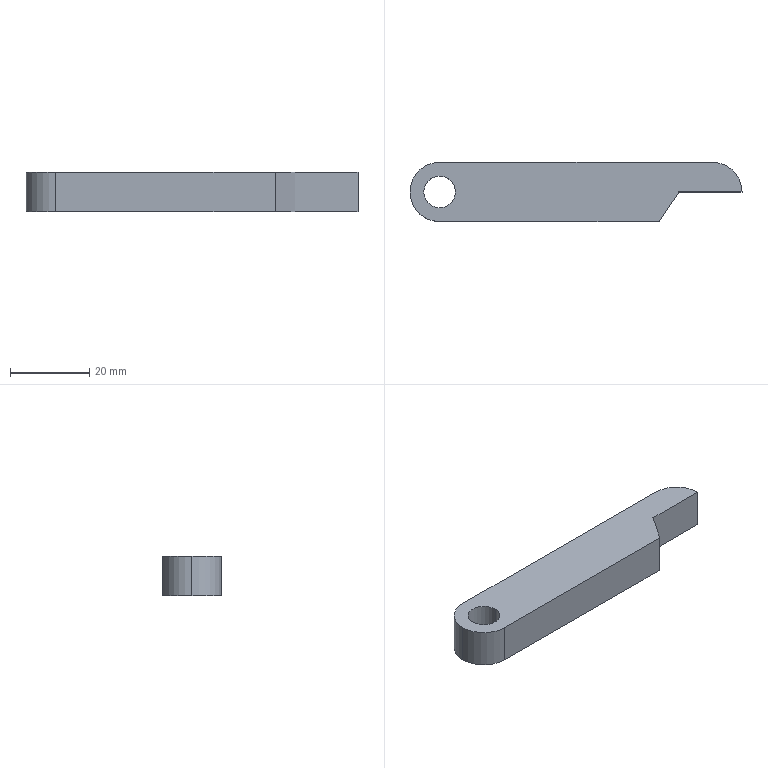Part | SolidWorks | features Extrusion 1 | 1 solid | 11 faces | box 84 x 15 x 10 mm | volume 10349 mm3 | plane 6 | cylinder 5 | commonest cylinder face diameters 15 x3 8 x2
STEP:
#1=CARTESIAN_POINT('',(-4.,0.,10.));
#2=VERTEX_POINT('',#1);
#3=CARTESIAN_POINT('',(4.,0.,10.));
#4=VERTEX_POINT('',#3);
#5=CARTESIAN_POINT('',(0.,0.,10.));
#6=DIRECTION('',(0.,0.,1.));
#7=DIRECTION('',(1.,0.,0.));
#8=AXIS2_PLACEMENT_3D('',#5,#6,#7);
#9=CIRCLE('',#8,4.);
#10=EDGE_CURVE('',#2,#4,#9,.T.);
#11=ORIENTED_EDGE('',*,*,#10,.T.);
#12=CARTESIAN_POINT('',(4.,0.,0.));
#13=VERTEX_POINT('',#12);
#14=CARTESIAN_POINT('',(4.,0.,10.));
#15=DIRECTION('',(0.,0.,-1.));
#16=VECTOR('',#15,1000.);
#17=LINE('',#14,#16);
#18=EDGE_CURVE('',#4,#13,#17,.T.);
#19=ORIENTED_EDGE('',*,*,#18,.T.);
#20=CARTESIAN_POINT('',(-4.,0.,0.));
#21=VERTEX_POINT('',#20);
#22=CARTESIAN_POINT('',(0.,0.,0.));
#23=DIRECTION('',(0.,0.,1.));
#24=DIRECTION('',(1.,0.,0.));
#25=AXIS2_PLACEMENT_3D('',#22,#23,#24);
#26=CIRCLE('',#25,4.);
#27=EDGE_CURVE('',#21,#13,#26,.T.);
#28=ORIENTED_EDGE('',*,*,#27,.F.);
#29=CARTESIAN_POINT('',(-4.,0.,10.));
#30=DIRECTION('',(0.,0.,-1.));
#31=VECTOR('',#30,1000.);
#32=LINE('',#29,#31);
#33=EDGE_CURVE('',#2,#21,#32,.T.);
#34=ORIENTED_EDGE('',*,*,#33,.F.);
#35=EDGE_LOOP('',(#11,#19,#28,#34));
#36=FACE_OUTER_BOUND('',#35,.T.);
#37=CARTESIAN_POINT('',(0.,0.,10.));
#38=DIRECTION('',(0.,0.,-1.));
#39=DIRECTION('',(-1.,0.,0.));
#40=AXIS2_PLACEMENT_3D('',#37,#38,#39);
#41=CYLINDRICAL_SURFACE('',#40,4.);
#42=ADVANCED_FACE('',(#36),#41,.F.);
#43=CARTESIAN_POINT('',(-7.5,0.,10.));
#44=VERTEX_POINT('',#43);
#45=CARTESIAN_POINT('',(0.,-7.5,10.));
#46=VERTEX_POINT('',#45);
#47=CARTESIAN_POINT('',(0.,0.,10.));
#48=DIRECTION('',(0.,0.,1.));
#49=DIRECTION('',(1.,0.,0.));
#50=AXIS2_PLACEMENT_3D('',#47,#48,#49);
#51=CIRCLE('',#50,7.5);
#52=EDGE_CURVE('',#44,#46,#51,.T.);
#53=ORIENTED_EDGE('',*,*,#52,.F.);
#54=CARTESIAN_POINT('',(-7.5,0.,0.));
#55=VERTEX_POINT('',#54);
#56=CARTESIAN_POINT('',(-7.5,0.,10.));
#57=DIRECTION('',(0.,0.,-1.));
#58=VECTOR('',#57,1000.);
#59=LINE('',#56,#58);
#60=EDGE_CURVE('',#44,#55,#59,.T.);
#61=ORIENTED_EDGE('',*,*,#60,.T.);
#62=CARTESIAN_POINT('',(0.,-7.5,0.));
#63=VERTEX_POINT('',#62);
#64=CARTESIAN_POINT('',(0.,0.,0.));
#65=DIRECTION('',(0.,0.,1.));
#66=DIRECTION('',(1.,0.,0.));
#67=AXIS2_PLACEMENT_3D('',#64,#65,#66);
#68=CIRCLE('',#67,7.5);
#69=EDGE_CURVE('',#55,#63,#68,.T.);
#70=ORIENTED_EDGE('',*,*,#69,.T.);
#71=CARTESIAN_POINT('',(0.,-7.5,10.));
#72=DIRECTION('',(0.,0.,-1.));
#73=VECTOR('',#72,1000.);
#74=LINE('',#71,#73);
#75=EDGE_CURVE('',#46,#63,#74,.T.);
#76=ORIENTED_EDGE('',*,*,#75,.F.);
#77=EDGE_LOOP('',(#53,#61,#70,#76));
#78=FACE_OUTER_BOUND('',#77,.T.);
#79=CARTESIAN_POINT('',(0.,0.,10.));
#80=DIRECTION('',(0.,0.,-1.));
#81=DIRECTION('',(-1.,0.,0.));
#82=AXIS2_PLACEMENT_3D('',#79,#80,#81);
#83=CYLINDRICAL_SURFACE('',#82,7.5);
#84=ADVANCED_FACE('',(#78),#83,.T.);
#85=CARTESIAN_POINT('',(55.536,-7.5,10.));
#86=VERTEX_POINT('',#85);
#87=CARTESIAN_POINT('',(60.5,0.,10.));
#88=VERTEX_POINT('',#87);
#89=CARTESIAN_POINT('',(55.536,-7.5,10.));
#90=DIRECTION('',(0.552,0.8339,0.));
#91=VECTOR('',#90,1000.);
#92=LINE('',#89,#91);
#93=EDGE_CURVE('',#86,#88,#92,.T.);
#94=ORIENTED_EDGE('',*,*,#93,.T.);
#95=CARTESIAN_POINT('',(76.5,0.,10.));
#96=VERTEX_POINT('',#95);
#97=CARTESIAN_POINT('',(60.5,0.,10.));
#98=DIRECTION('',(1.,0.,0.));
#99=VECTOR('',#98,1000.);
#100=LINE('',#97,#99);
#101=EDGE_CURVE('',#88,#96,#100,.T.);
#102=ORIENTED_EDGE('',*,*,#101,.T.);
#103=CARTESIAN_POINT('',(69.,7.5,10.));
#104=VERTEX_POINT('',#103);
#105=CARTESIAN_POINT('',(69.,0.,10.));
#106=DIRECTION('',(0.,0.,1.));
#107=DIRECTION('',(1.,0.,0.));
#108=AXIS2_PLACEMENT_3D('',#105,#106,#107);
#109=CIRCLE('',#108,7.5);
#110=EDGE_CURVE('',#96,#104,#109,.T.);
#111=ORIENTED_EDGE('',*,*,#110,.T.);
#112=CARTESIAN_POINT('',(0.,7.5,10.));
#113=VERTEX_POINT('',#112);
#114=CARTESIAN_POINT('',(0.,7.5,10.));
#115=DIRECTION('',(-1.,0.,0.));
#116=VECTOR('',#115,1000.);
#117=LINE('',#114,#116);
#118=EDGE_CURVE('',#104,#113,#117,.T.);
#119=ORIENTED_EDGE('',*,*,#118,.T.);
#120=CARTESIAN_POINT('',(0.,0.,10.));
#121=DIRECTION('',(0.,0.,1.));
#122=DIRECTION('',(1.,0.,0.));
#123=AXIS2_PLACEMENT_3D('',#120,#121,#122);
#124=CIRCLE('',#123,7.5);
#125=EDGE_CURVE('',#113,#44,#124,.T.);
#126=ORIENTED_EDGE('',*,*,#125,.T.);
#127=ORIENTED_EDGE('',*,*,#52,.T.);
#128=CARTESIAN_POINT('',(55.536,-7.5,10.));
#129=DIRECTION('',(1.,0.,0.));
#130=VECTOR('',#129,1000.);
#131=LINE('',#128,#130);
#132=EDGE_CURVE('',#46,#86,#131,.T.);
#133=ORIENTED_EDGE('',*,*,#132,.T.);
#134=EDGE_LOOP('',(#94,#102,#111,#119,#126,#127,#133));
#135=FACE_OUTER_BOUND('',#134,.T.);
#136=ORIENTED_EDGE('',*,*,#10,.F.);
#137=CARTESIAN_POINT('',(0.,0.,10.));
#138=DIRECTION('',(0.,0.,1.));
#139=DIRECTION('',(1.,0.,0.));
#140=AXIS2_PLACEMENT_3D('',#137,#138,#139);
#141=CIRCLE('',#140,4.);
#142=EDGE_CURVE('',#4,#2,#141,.T.);
#143=ORIENTED_EDGE('',*,*,#142,.F.);
#144=EDGE_LOOP('',(#136,#143));
#145=FACE_BOUND('',#144,.T.);
#146=CARTESIAN_POINT('',(69.,0.,10.));
#147=DIRECTION('',(0.,0.,1.));
#148=DIRECTION('',(1.,0.,0.));
#149=AXIS2_PLACEMENT_3D('',#146,#147,#148);
#150=PLANE('',#149);
#151=ADVANCED_FACE('',(#135,#145),#150,.T.);
#152=CARTESIAN_POINT('',(55.536,-7.5,0.));
#153=VERTEX_POINT('',#152);
#154=CARTESIAN_POINT('',(60.5,0.,0.));
#155=VERTEX_POINT('',#154);
#156=CARTESIAN_POINT('',(55.536,-7.5,0.));
#157=DIRECTION('',(0.552,0.8339,0.));
#158=VECTOR('',#157,1000.);
#159=LINE('',#156,#158);
#160=EDGE_CURVE('',#153,#155,#159,.T.);
#161=ORIENTED_EDGE('',*,*,#160,.F.);
#162=CARTESIAN_POINT('',(55.536,-7.5,0.));
#163=DIRECTION('',(1.,0.,0.));
#164=VECTOR('',#163,1000.);
#165=LINE('',#162,#164);
#166=EDGE_CURVE('',#63,#153,#165,.T.);
#167=ORIENTED_EDGE('',*,*,#166,.F.);
#168=ORIENTED_EDGE('',*,*,#69,.F.);
#169=CARTESIAN_POINT('',(0.,7.5,0.));
#170=VERTEX_POINT('',#169);
#171=CARTESIAN_POINT('',(0.,0.,0.));
#172=DIRECTION('',(0.,0.,1.));
#173=DIRECTION('',(1.,0.,0.));
#174=AXIS2_PLACEMENT_3D('',#171,#172,#173);
#175=CIRCLE('',#174,7.5);
#176=EDGE_CURVE('',#170,#55,#175,.T.);
#177=ORIENTED_EDGE('',*,*,#176,.F.);
#178=CARTESIAN_POINT('',(69.,7.5,0.));
#179=VERTEX_POINT('',#178);
#180=CARTESIAN_POINT('',(0.,7.5,0.));
#181=DIRECTION('',(-1.,0.,0.));
#182=VECTOR('',#181,1000.);
#183=LINE('',#180,#182);
#184=EDGE_CURVE('',#179,#170,#183,.T.);
#185=ORIENTED_EDGE('',*,*,#184,.F.);
#186=CARTESIAN_POINT('',(76.5,0.,0.));
#187=VERTEX_POINT('',#186);
#188=CARTESIAN_POINT('',(69.,0.,0.));
#189=DIRECTION('',(0.,0.,1.));
#190=DIRECTION('',(1.,0.,0.));
#191=AXIS2_PLACEMENT_3D('',#188,#189,#190);
#192=CIRCLE('',#191,7.5);
#193=EDGE_CURVE('',#187,#179,#192,.T.);
#194=ORIENTED_EDGE('',*,*,#193,.F.);
#195=CARTESIAN_POINT('',(60.5,0.,0.));
#196=DIRECTION('',(1.,0.,0.));
#197=VECTOR('',#196,1000.);
#198=LINE('',#195,#197);
#199=EDGE_CURVE('',#155,#187,#198,.T.);
#200=ORIENTED_EDGE('',*,*,#199,.F.);
#201=EDGE_LOOP('',(#161,#167,#168,#177,#185,#194,#200));
#202=FACE_OUTER_BOUND('',#201,.T.);
#203=ORIENTED_EDGE('',*,*,#27,.T.);
#204=CARTESIAN_POINT('',(0.,0.,0.));
#205=DIRECTION('',(0.,0.,1.));
#206=DIRECTION('',(1.,0.,0.));
#207=AXIS2_PLACEMENT_3D('',#204,#205,#206);
#208=CIRCLE('',#207,4.);
#209=EDGE_CURVE('',#13,#21,#208,.T.);
#210=ORIENTED_EDGE('',*,*,#209,.T.);
#211=EDGE_LOOP('',(#203,#210));
#212=FACE_BOUND('',#211,.T.);
#213=CARTESIAN_POINT('',(69.,0.,0.));
#214=DIRECTION('',(0.,0.,1.));
#215=DIRECTION('',(1.,0.,0.));
#216=AXIS2_PLACEMENT_3D('',#213,#214,#215);
#217=PLANE('',#216);
#218=ADVANCED_FACE('',(#202,#212),#217,.F.);
#219=ORIENTED_EDGE('',*,*,#160,.T.);
#220=CARTESIAN_POINT('',(60.5,0.,10.));
#221=DIRECTION('',(0.,0.,-1.));
#222=VECTOR('',#221,1000.);
#223=LINE('',#220,#222);
#224=EDGE_CURVE('',#88,#155,#223,.T.);
#225=ORIENTED_EDGE('',*,*,#224,.F.);
#226=ORIENTED_EDGE('',*,*,#93,.F.);
#227=CARTESIAN_POINT('',(55.536,-7.5,10.));
#228=DIRECTION('',(0.,0.,-1.));
#229=VECTOR('',#228,1000.);
#230=LINE('',#227,#229);
#231=EDGE_CURVE('',#86,#153,#230,.T.);
#232=ORIENTED_EDGE('',*,*,#231,.T.);
#233=EDGE_LOOP('',(#219,#225,#226,#232));
#234=FACE_OUTER_BOUND('',#233,.T.);
#235=CARTESIAN_POINT('',(55.536,-7.5,10.));
#236=DIRECTION('',(-0.8339,0.552,0.));
#237=DIRECTION('',(-0.552,-0.8339,0.));
#238=AXIS2_PLACEMENT_3D('',#235,#236,#237);
#239=PLANE('',#238);
#240=ADVANCED_FACE('',(#234),#239,.F.);
#241=ORIENTED_EDGE('',*,*,#199,.T.);
#242=CARTESIAN_POINT('',(76.5,0.,10.));
#243=DIRECTION('',(0.,0.,-1.));
#244=VECTOR('',#243,1000.);
#245=LINE('',#242,#244);
#246=EDGE_CURVE('',#96,#187,#245,.T.);
#247=ORIENTED_EDGE('',*,*,#246,.F.);
#248=ORIENTED_EDGE('',*,*,#101,.F.);
#249=ORIENTED_EDGE('',*,*,#224,.T.);
#250=EDGE_LOOP('',(#241,#247,#248,#249));
#251=FACE_OUTER_BOUND('',#250,.T.);
#252=CARTESIAN_POINT('',(60.5,0.,10.));
#253=DIRECTION('',(0.,1.,0.));
#254=DIRECTION('',(0.,0.,1.));
#255=AXIS2_PLACEMENT_3D('',#252,#253,#254);
#256=PLANE('',#255);
#257=ADVANCED_FACE('',(#251),#256,.F.);
#258=ORIENTED_EDGE('',*,*,#193,.T.);
#259=CARTESIAN_POINT('',(69.,7.5,10.));
#260=DIRECTION('',(0.,0.,-1.));
#261=VECTOR('',#260,1000.);
#262=LINE('',#259,#261);
#263=EDGE_CURVE('',#104,#179,#262,.T.);
#264=ORIENTED_EDGE('',*,*,#263,.F.);
#265=ORIENTED_EDGE('',*,*,#110,.F.);
#266=ORIENTED_EDGE('',*,*,#246,.T.);
#267=EDGE_LOOP('',(#258,#264,#265,#266));
#268=FACE_OUTER_BOUND('',#267,.T.);
#269=CARTESIAN_POINT('',(69.,0.,10.));
#270=DIRECTION('',(0.,0.,-1.));
#271=DIRECTION('',(-1.,0.,0.));
#272=AXIS2_PLACEMENT_3D('',#269,#270,#271);
#273=CYLINDRICAL_SURFACE('',#272,7.5);
#274=ADVANCED_FACE('',(#268),#273,.T.);
#275=ORIENTED_EDGE('',*,*,#184,.T.);
#276=CARTESIAN_POINT('',(0.,7.5,10.));
#277=DIRECTION('',(0.,0.,-1.));
#278=VECTOR('',#277,1000.);
#279=LINE('',#276,#278);
#280=EDGE_CURVE('',#113,#170,#279,.T.);
#281=ORIENTED_EDGE('',*,*,#280,.F.);
#282=ORIENTED_EDGE('',*,*,#118,.F.);
#283=ORIENTED_EDGE('',*,*,#263,.T.);
#284=EDGE_LOOP('',(#275,#281,#282,#283));
#285=FACE_OUTER_BOUND('',#284,.T.);
#286=CARTESIAN_POINT('',(0.,7.5,10.));
#287=DIRECTION('',(0.,-1.,0.));
#288=DIRECTION('',(1.,0.,0.));
#289=AXIS2_PLACEMENT_3D('',#286,#287,#288);
#290=PLANE('',#289);
#291=ADVANCED_FACE('',(#285),#290,.F.);
#292=ORIENTED_EDGE('',*,*,#60,.F.);
#293=ORIENTED_EDGE('',*,*,#125,.F.);
#294=ORIENTED_EDGE('',*,*,#280,.T.);
#295=ORIENTED_EDGE('',*,*,#176,.T.);
#296=EDGE_LOOP('',(#292,#293,#294,#295));
#297=FACE_OUTER_BOUND('',#296,.T.);
#298=CARTESIAN_POINT('',(0.,0.,10.));
#299=DIRECTION('',(0.,0.,-1.));
#300=DIRECTION('',(-1.,0.,0.));
#301=AXIS2_PLACEMENT_3D('',#298,#299,#300);
#302=CYLINDRICAL_SURFACE('',#301,7.5);
#303=ADVANCED_FACE('',(#297),#302,.T.);
#304=ORIENTED_EDGE('',*,*,#166,.T.);
#305=ORIENTED_EDGE('',*,*,#231,.F.);
#306=ORIENTED_EDGE('',*,*,#132,.F.);
#307=ORIENTED_EDGE('',*,*,#75,.T.);
#308=EDGE_LOOP('',(#304,#305,#306,#307));
#309=FACE_OUTER_BOUND('',#308,.T.);
#310=CARTESIAN_POINT('',(55.536,-7.5,10.));
#311=DIRECTION('',(0.,1.,0.));
#312=DIRECTION('',(-1.,0.,0.));
#313=AXIS2_PLACEMENT_3D('',#310,#311,#312);
#314=PLANE('',#313);
#315=ADVANCED_FACE('',(#309),#314,.F.);
#316=ORIENTED_EDGE('',*,*,#18,.F.);
#317=ORIENTED_EDGE('',*,*,#142,.T.);
#318=ORIENTED_EDGE('',*,*,#33,.T.);
#319=ORIENTED_EDGE('',*,*,#209,.F.);
#320=EDGE_LOOP('',(#316,#317,#318,#319));
#321=FACE_OUTER_BOUND('',#320,.T.);
#322=CARTESIAN_POINT('',(0.,0.,10.));
#323=DIRECTION('',(0.,0.,-1.));
#324=DIRECTION('',(-1.,0.,0.));
#325=AXIS2_PLACEMENT_3D('',#322,#323,#324);
#326=CYLINDRICAL_SURFACE('',#325,4.);
#327=ADVANCED_FACE('',(#321),#326,.F.);
#328=CLOSED_SHELL('',(#42,#84,#151,#218,#240,#257,#274,#291,#303,#315,#327));
#329=MANIFOLD_SOLID_BREP('',#328);
#330=CARTESIAN_POINT('',(0.,0.,0.));
#331=DIRECTION('',(0.,0.,1.));
#332=DIRECTION('',(1.,0.,0.));
#333=AXIS2_PLACEMENT_3D('',#330,#331,#332);
#334=(LENGTH_UNIT()NAMED_UNIT(*)SI_UNIT(.MILLI.,.METRE.));
#335=UNCERTAINTY_MEASURE_WITH_UNIT(LENGTH_MEASURE(0.00001),#334,'','');
#336=(NAMED_UNIT(*)PLANE_ANGLE_UNIT()SI_UNIT($,.RADIAN.));
#337=(NAMED_UNIT(*)SI_UNIT($,.STERADIAN.)SOLID_ANGLE_UNIT());
#338=(GEOMETRIC_REPRESENTATION_CONTEXT(3)GLOBAL_UNCERTAINTY_ASSIGNED_CONTEXT((#335))GLOBAL_UNIT_ASSIGNED_CONTEXT((#334,#336,#337))REPRESENTATION_CONTEXT('',''));
#339=ADVANCED_BREP_SHAPE_REPRESENTATION('',(#329,#333),#338);